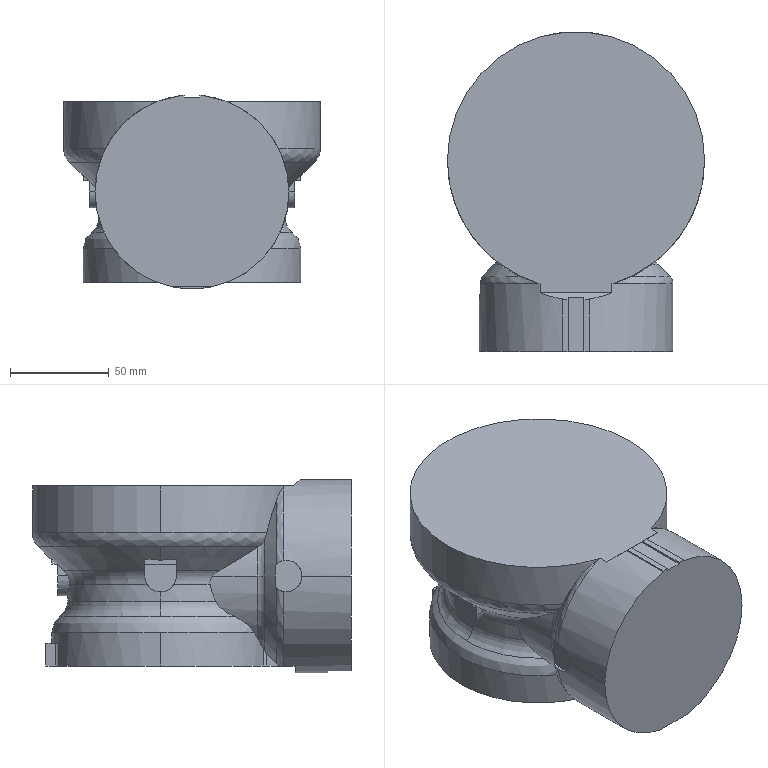Part | STEP file | Link5 | 1 solid | 99 faces | box 130 x 161.5 x 98 mm | volume 1253292 mm3 | plane 52 | cylinder 26 | torus 10 | cone 6 | spline 5 | commonest cylinder face diameters 16 x6 4 x4 80 x3 94 x3 98 x3 110 x3